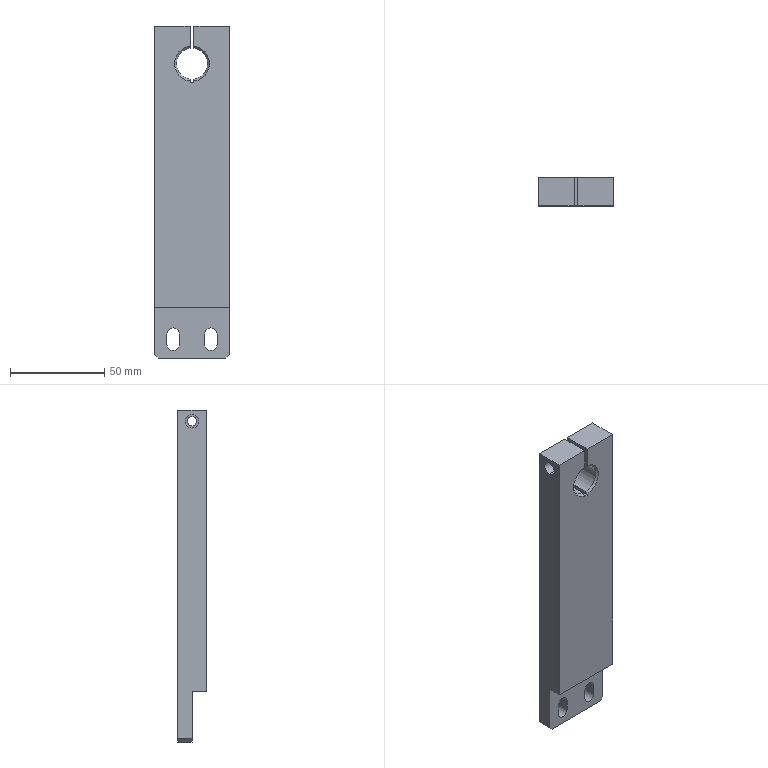Part | STEP file | 0229_218_Arm | 1 solid | 34 faces | box 40 x 15 x 176.5 mm | volume 91943 mm3 | plane 20 | cylinder 12 | cone 2 | commonest cylinder face diameters 6.6 x6 5 x2 7 x2 16.6 x2